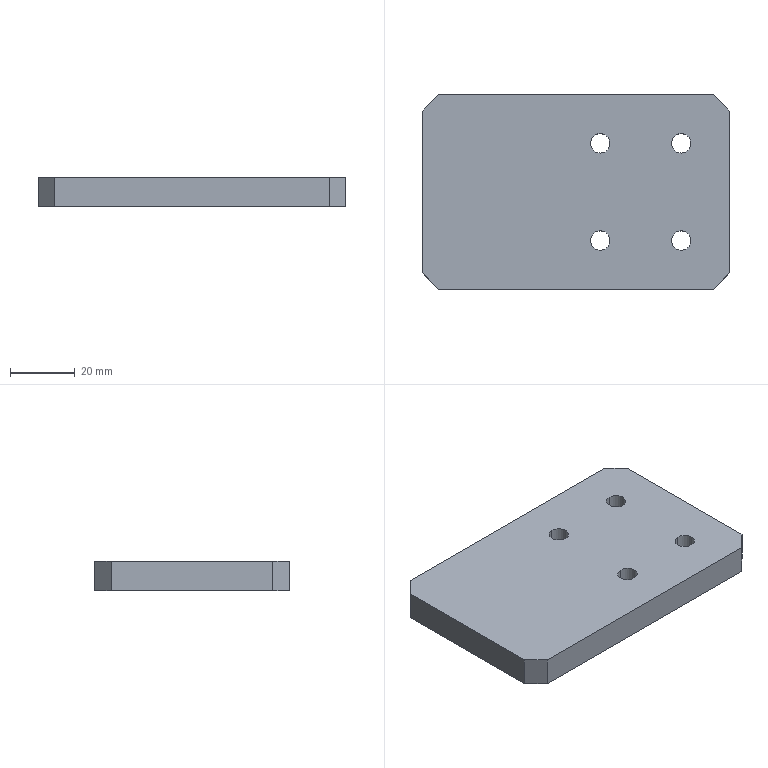Part | STEP file | [12] | 1 solid | 18 faces | box 95 x 60 x 9 mm | volume 49832 mm3 | plane 10 | cylinder 8 | commonest cylinder face diameters 6 x8